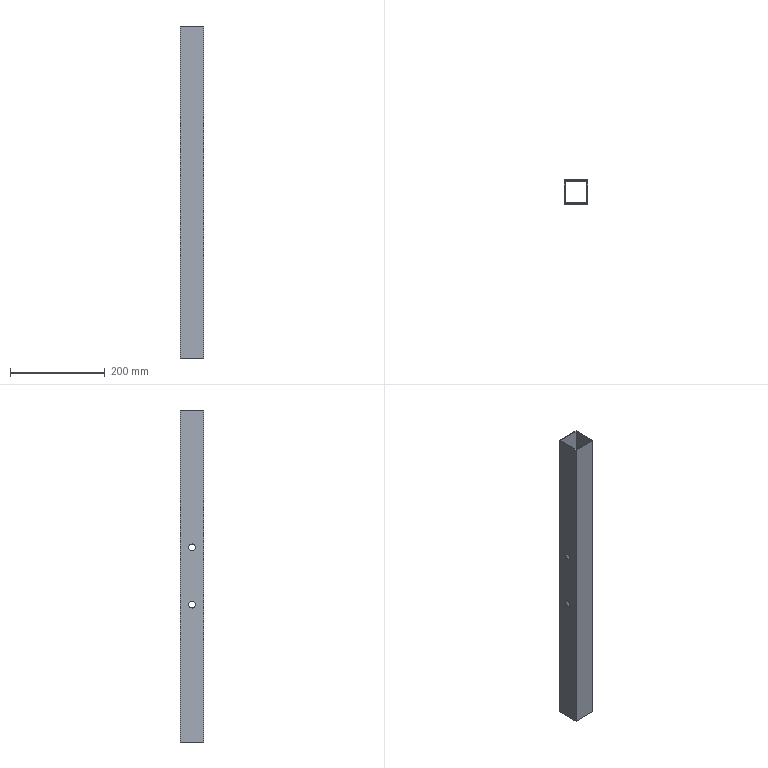Part | SolidWorks | features Extrusion 1, ICE 1 | 1 solid | 18 faces | box 50 x 50 x 700 mm | volume 267568 mm3 | plane 10 | cylinder 8 | commonest cylinder face diameters 14 x8
STEP:
#1=CARTESIAN_POINT('',(25.,0.,403.5));
#2=VERTEX_POINT('',#1);
#3=CARTESIAN_POINT('',(25.,0.,417.5));
#4=VERTEX_POINT('',#3);
#5=CARTESIAN_POINT('',(25.,0.,410.5));
#6=DIRECTION('',(-1.,0.,0.));
#7=DIRECTION('',(0.,0.,-1.));
#8=AXIS2_PLACEMENT_3D('',#5,#6,#7);
#9=CIRCLE('',#8,7.);
#10=EDGE_CURVE('',#2,#4,#9,.T.);
#11=ORIENTED_EDGE('',*,*,#10,.F.);
#12=CARTESIAN_POINT('',(23.,0.,403.5));
#13=VERTEX_POINT('',#12);
#14=CARTESIAN_POINT('',(25.,0.,403.5));
#15=DIRECTION('',(-1.,0.,0.));
#16=VECTOR('',#15,1000.);
#17=LINE('',#14,#16);
#18=EDGE_CURVE('',#2,#13,#17,.T.);
#19=ORIENTED_EDGE('',*,*,#18,.T.);
#20=CARTESIAN_POINT('',(23.,0.,417.5));
#21=VERTEX_POINT('',#20);
#22=CARTESIAN_POINT('',(23.,0.,410.5));
#23=DIRECTION('',(-1.,0.,0.));
#24=DIRECTION('',(0.,0.,1.));
#25=AXIS2_PLACEMENT_3D('',#22,#23,#24);
#26=CIRCLE('',#25,7.);
#27=EDGE_CURVE('',#13,#21,#26,.T.);
#28=ORIENTED_EDGE('',*,*,#27,.T.);
#29=CARTESIAN_POINT('',(25.,0.,417.5));
#30=DIRECTION('',(-1.,0.,0.));
#31=VECTOR('',#30,1000.);
#32=LINE('',#29,#31);
#33=EDGE_CURVE('',#4,#21,#32,.T.);
#34=ORIENTED_EDGE('',*,*,#33,.F.);
#35=EDGE_LOOP('',(#11,#19,#28,#34));
#36=FACE_OUTER_BOUND('',#35,.T.);
#37=CARTESIAN_POINT('',(25.,0.,410.5));
#38=DIRECTION('',(-1.,0.,0.));
#39=DIRECTION('',(0.,0.,1.));
#40=AXIS2_PLACEMENT_3D('',#37,#38,#39);
#41=CYLINDRICAL_SURFACE('',#40,7.);
#42=ADVANCED_FACE('',(#36),#41,.F.);
#43=CARTESIAN_POINT('',(-23.,0.,417.5));
#44=VERTEX_POINT('',#43);
#45=CARTESIAN_POINT('',(-23.,0.,403.5));
#46=VERTEX_POINT('',#45);
#47=CARTESIAN_POINT('',(-23.,0.,410.5));
#48=DIRECTION('',(1.,0.,0.));
#49=DIRECTION('',(0.,0.,-1.));
#50=AXIS2_PLACEMENT_3D('',#47,#48,#49);
#51=CIRCLE('',#50,7.);
#52=EDGE_CURVE('',#44,#46,#51,.T.);
#53=ORIENTED_EDGE('',*,*,#52,.T.);
#54=CARTESIAN_POINT('',(-25.,0.,403.5));
#55=VERTEX_POINT('',#54);
#56=CARTESIAN_POINT('',(25.,0.,403.5));
#57=DIRECTION('',(-1.,0.,0.));
#58=VECTOR('',#57,1000.);
#59=LINE('',#56,#58);
#60=EDGE_CURVE('',#46,#55,#59,.T.);
#61=ORIENTED_EDGE('',*,*,#60,.T.);
#62=CARTESIAN_POINT('',(-25.,0.,417.5));
#63=VERTEX_POINT('',#62);
#64=CARTESIAN_POINT('',(-25.,0.,410.5));
#65=DIRECTION('',(-1.,0.,0.));
#66=DIRECTION('',(0.,0.,-1.));
#67=AXIS2_PLACEMENT_3D('',#64,#65,#66);
#68=CIRCLE('',#67,7.);
#69=EDGE_CURVE('',#55,#63,#68,.T.);
#70=ORIENTED_EDGE('',*,*,#69,.T.);
#71=CARTESIAN_POINT('',(25.,0.,417.5));
#72=DIRECTION('',(-1.,0.,0.));
#73=VECTOR('',#72,1000.);
#74=LINE('',#71,#73);
#75=EDGE_CURVE('',#44,#63,#74,.T.);
#76=ORIENTED_EDGE('',*,*,#75,.F.);
#77=EDGE_LOOP('',(#53,#61,#70,#76));
#78=FACE_OUTER_BOUND('',#77,.T.);
#79=CARTESIAN_POINT('',(25.,0.,410.5));
#80=DIRECTION('',(-1.,0.,0.));
#81=DIRECTION('',(0.,0.,1.));
#82=AXIS2_PLACEMENT_3D('',#79,#80,#81);
#83=CYLINDRICAL_SURFACE('',#82,7.);
#84=ADVANCED_FACE('',(#78),#83,.F.);
#85=CARTESIAN_POINT('',(25.,0.,282.5));
#86=VERTEX_POINT('',#85);
#87=CARTESIAN_POINT('',(25.,0.,296.5));
#88=VERTEX_POINT('',#87);
#89=CARTESIAN_POINT('',(25.,0.,289.5));
#90=DIRECTION('',(-1.,0.,0.));
#91=DIRECTION('',(0.,0.,1.));
#92=AXIS2_PLACEMENT_3D('',#89,#90,#91);
#93=CIRCLE('',#92,7.);
#94=EDGE_CURVE('',#86,#88,#93,.T.);
#95=ORIENTED_EDGE('',*,*,#94,.F.);
#96=CARTESIAN_POINT('',(23.,0.,282.5));
#97=VERTEX_POINT('',#96);
#98=CARTESIAN_POINT('',(25.,0.,282.5));
#99=DIRECTION('',(-1.,0.,0.));
#100=VECTOR('',#99,1000.);
#101=LINE('',#98,#100);
#102=EDGE_CURVE('',#86,#97,#101,.T.);
#103=ORIENTED_EDGE('',*,*,#102,.T.);
#104=CARTESIAN_POINT('',(23.,0.,296.5));
#105=VERTEX_POINT('',#104);
#106=CARTESIAN_POINT('',(23.,0.,289.5));
#107=DIRECTION('',(-1.,0.,0.));
#108=DIRECTION('',(0.,0.,1.));
#109=AXIS2_PLACEMENT_3D('',#106,#107,#108);
#110=CIRCLE('',#109,7.);
#111=EDGE_CURVE('',#97,#105,#110,.T.);
#112=ORIENTED_EDGE('',*,*,#111,.T.);
#113=CARTESIAN_POINT('',(25.,0.,296.5));
#114=DIRECTION('',(-1.,0.,0.));
#115=VECTOR('',#114,1000.);
#116=LINE('',#113,#115);
#117=EDGE_CURVE('',#88,#105,#116,.T.);
#118=ORIENTED_EDGE('',*,*,#117,.F.);
#119=EDGE_LOOP('',(#95,#103,#112,#118));
#120=FACE_OUTER_BOUND('',#119,.T.);
#121=CARTESIAN_POINT('',(25.,0.,289.5));
#122=DIRECTION('',(-1.,0.,0.));
#123=DIRECTION('',(0.,0.,1.));
#124=AXIS2_PLACEMENT_3D('',#121,#122,#123);
#125=CYLINDRICAL_SURFACE('',#124,7.);
#126=ADVANCED_FACE('',(#120),#125,.F.);
#127=CARTESIAN_POINT('',(-23.,0.,296.5));
#128=VERTEX_POINT('',#127);
#129=CARTESIAN_POINT('',(-23.,0.,282.5));
#130=VERTEX_POINT('',#129);
#131=CARTESIAN_POINT('',(-23.,0.,289.5));
#132=DIRECTION('',(1.,0.,0.));
#133=DIRECTION('',(0.,0.,-1.));
#134=AXIS2_PLACEMENT_3D('',#131,#132,#133);
#135=CIRCLE('',#134,7.);
#136=EDGE_CURVE('',#128,#130,#135,.T.);
#137=ORIENTED_EDGE('',*,*,#136,.T.);
#138=CARTESIAN_POINT('',(-25.,0.,282.5));
#139=VERTEX_POINT('',#138);
#140=CARTESIAN_POINT('',(25.,0.,282.5));
#141=DIRECTION('',(-1.,0.,0.));
#142=VECTOR('',#141,1000.);
#143=LINE('',#140,#142);
#144=EDGE_CURVE('',#130,#139,#143,.T.);
#145=ORIENTED_EDGE('',*,*,#144,.T.);
#146=CARTESIAN_POINT('',(-25.,0.,296.5));
#147=VERTEX_POINT('',#146);
#148=CARTESIAN_POINT('',(-25.,0.,289.5));
#149=DIRECTION('',(-1.,0.,0.));
#150=DIRECTION('',(0.,0.,1.));
#151=AXIS2_PLACEMENT_3D('',#148,#149,#150);
#152=CIRCLE('',#151,7.);
#153=EDGE_CURVE('',#139,#147,#152,.T.);
#154=ORIENTED_EDGE('',*,*,#153,.T.);
#155=CARTESIAN_POINT('',(25.,0.,296.5));
#156=DIRECTION('',(-1.,0.,0.));
#157=VECTOR('',#156,1000.);
#158=LINE('',#155,#157);
#159=EDGE_CURVE('',#128,#147,#158,.T.);
#160=ORIENTED_EDGE('',*,*,#159,.F.);
#161=EDGE_LOOP('',(#137,#145,#154,#160));
#162=FACE_OUTER_BOUND('',#161,.T.);
#163=CARTESIAN_POINT('',(25.,0.,289.5));
#164=DIRECTION('',(-1.,0.,0.));
#165=DIRECTION('',(0.,0.,1.));
#166=AXIS2_PLACEMENT_3D('',#163,#164,#165);
#167=CYLINDRICAL_SURFACE('',#166,7.);
#168=ADVANCED_FACE('',(#162),#167,.F.);
#169=CARTESIAN_POINT('',(25.,-25.,700.));
#170=VERTEX_POINT('',#169);
#171=CARTESIAN_POINT('',(25.,25.,700.));
#172=VERTEX_POINT('',#171);
#173=CARTESIAN_POINT('',(25.,-25.,700.));
#174=DIRECTION('',(0.,1.,0.));
#175=VECTOR('',#174,1000.);
#176=LINE('',#173,#175);
#177=EDGE_CURVE('',#170,#172,#176,.T.);
#178=ORIENTED_EDGE('',*,*,#177,.T.);
#179=CARTESIAN_POINT('',(-25.,25.,700.));
#180=VERTEX_POINT('',#179);
#181=CARTESIAN_POINT('',(-25.,25.,700.));
#182=DIRECTION('',(-1.,0.,0.));
#183=VECTOR('',#182,1000.);
#184=LINE('',#181,#183);
#185=EDGE_CURVE('',#172,#180,#184,.T.);
#186=ORIENTED_EDGE('',*,*,#185,.T.);
#187=CARTESIAN_POINT('',(-25.,-25.,700.));
#188=VERTEX_POINT('',#187);
#189=CARTESIAN_POINT('',(-25.,-25.,700.));
#190=DIRECTION('',(0.,-1.,0.));
#191=VECTOR('',#190,1000.);
#192=LINE('',#189,#191);
#193=EDGE_CURVE('',#180,#188,#192,.T.);
#194=ORIENTED_EDGE('',*,*,#193,.T.);
#195=CARTESIAN_POINT('',(-25.,-25.,700.));
#196=DIRECTION('',(1.,0.,0.));
#197=VECTOR('',#196,1000.);
#198=LINE('',#195,#197);
#199=EDGE_CURVE('',#188,#170,#198,.T.);
#200=ORIENTED_EDGE('',*,*,#199,.T.);
#201=EDGE_LOOP('',(#178,#186,#194,#200));
#202=FACE_OUTER_BOUND('',#201,.T.);
#203=CARTESIAN_POINT('',(23.,-23.,700.));
#204=VERTEX_POINT('',#203);
#205=CARTESIAN_POINT('',(23.,23.,700.));
#206=VERTEX_POINT('',#205);
#207=CARTESIAN_POINT('',(23.,-23.,700.));
#208=DIRECTION('',(0.,1.,0.));
#209=VECTOR('',#208,1000.);
#210=LINE('',#207,#209);
#211=EDGE_CURVE('',#204,#206,#210,.T.);
#212=ORIENTED_EDGE('',*,*,#211,.F.);
#213=CARTESIAN_POINT('',(-23.,-23.,700.));
#214=VERTEX_POINT('',#213);
#215=CARTESIAN_POINT('',(-23.,-23.,700.));
#216=DIRECTION('',(1.,0.,0.));
#217=VECTOR('',#216,1000.);
#218=LINE('',#215,#217);
#219=EDGE_CURVE('',#214,#204,#218,.T.);
#220=ORIENTED_EDGE('',*,*,#219,.F.);
#221=CARTESIAN_POINT('',(-23.,23.,700.));
#222=VERTEX_POINT('',#221);
#223=CARTESIAN_POINT('',(-23.,-23.,700.));
#224=DIRECTION('',(0.,-1.,0.));
#225=VECTOR('',#224,1000.);
#226=LINE('',#223,#225);
#227=EDGE_CURVE('',#222,#214,#226,.T.);
#228=ORIENTED_EDGE('',*,*,#227,.F.);
#229=CARTESIAN_POINT('',(-23.,23.,700.));
#230=DIRECTION('',(-1.,0.,0.));
#231=VECTOR('',#230,1000.);
#232=LINE('',#229,#231);
#233=EDGE_CURVE('',#206,#222,#232,.T.);
#234=ORIENTED_EDGE('',*,*,#233,.F.);
#235=EDGE_LOOP('',(#212,#220,#228,#234));
#236=FACE_BOUND('',#235,.T.);
#237=CARTESIAN_POINT('',(0.,0.,700.));
#238=DIRECTION('',(0.,0.,-1.));
#239=DIRECTION('',(-1.,0.,0.));
#240=AXIS2_PLACEMENT_3D('',#237,#238,#239);
#241=PLANE('',#240);
#242=ADVANCED_FACE('',(#202,#236),#241,.F.);
#243=CARTESIAN_POINT('',(25.,-25.,0.));
#244=VERTEX_POINT('',#243);
#245=CARTESIAN_POINT('',(25.,25.,0.));
#246=VERTEX_POINT('',#245);
#247=CARTESIAN_POINT('',(25.,-25.,0.));
#248=DIRECTION('',(0.,1.,0.));
#249=VECTOR('',#248,1000.);
#250=LINE('',#247,#249);
#251=EDGE_CURVE('',#244,#246,#250,.T.);
#252=ORIENTED_EDGE('',*,*,#251,.F.);
#253=CARTESIAN_POINT('',(-25.,-25.,0.));
#254=VERTEX_POINT('',#253);
#255=CARTESIAN_POINT('',(-25.,-25.,0.));
#256=DIRECTION('',(1.,0.,0.));
#257=VECTOR('',#256,1000.);
#258=LINE('',#255,#257);
#259=EDGE_CURVE('',#254,#244,#258,.T.);
#260=ORIENTED_EDGE('',*,*,#259,.F.);
#261=CARTESIAN_POINT('',(-25.,25.,0.));
#262=VERTEX_POINT('',#261);
#263=CARTESIAN_POINT('',(-25.,-25.,0.));
#264=DIRECTION('',(0.,-1.,0.));
#265=VECTOR('',#264,1000.);
#266=LINE('',#263,#265);
#267=EDGE_CURVE('',#262,#254,#266,.T.);
#268=ORIENTED_EDGE('',*,*,#267,.F.);
#269=CARTESIAN_POINT('',(-25.,25.,0.));
#270=DIRECTION('',(-1.,0.,0.));
#271=VECTOR('',#270,1000.);
#272=LINE('',#269,#271);
#273=EDGE_CURVE('',#246,#262,#272,.T.);
#274=ORIENTED_EDGE('',*,*,#273,.F.);
#275=EDGE_LOOP('',(#252,#260,#268,#274));
#276=FACE_OUTER_BOUND('',#275,.T.);
#277=CARTESIAN_POINT('',(-23.,-23.,0.));
#278=VERTEX_POINT('',#277);
#279=CARTESIAN_POINT('',(23.,-23.,0.));
#280=VERTEX_POINT('',#279);
#281=CARTESIAN_POINT('',(-23.,-23.,0.));
#282=DIRECTION('',(1.,0.,0.));
#283=VECTOR('',#282,1000.);
#284=LINE('',#281,#283);
#285=EDGE_CURVE('',#278,#280,#284,.T.);
#286=ORIENTED_EDGE('',*,*,#285,.T.);
#287=CARTESIAN_POINT('',(23.,23.,0.));
#288=VERTEX_POINT('',#287);
#289=CARTESIAN_POINT('',(23.,-23.,0.));
#290=DIRECTION('',(0.,1.,0.));
#291=VECTOR('',#290,1000.);
#292=LINE('',#289,#291);
#293=EDGE_CURVE('',#280,#288,#292,.T.);
#294=ORIENTED_EDGE('',*,*,#293,.T.);
#295=CARTESIAN_POINT('',(-23.,23.,0.));
#296=VERTEX_POINT('',#295);
#297=CARTESIAN_POINT('',(-23.,23.,0.));
#298=DIRECTION('',(-1.,0.,0.));
#299=VECTOR('',#298,1000.);
#300=LINE('',#297,#299);
#301=EDGE_CURVE('',#288,#296,#300,.T.);
#302=ORIENTED_EDGE('',*,*,#301,.T.);
#303=CARTESIAN_POINT('',(-23.,-23.,0.));
#304=DIRECTION('',(0.,-1.,0.));
#305=VECTOR('',#304,1000.);
#306=LINE('',#303,#305);
#307=EDGE_CURVE('',#296,#278,#306,.T.);
#308=ORIENTED_EDGE('',*,*,#307,.T.);
#309=EDGE_LOOP('',(#286,#294,#302,#308));
#310=FACE_BOUND('',#309,.T.);
#311=CARTESIAN_POINT('',(0.,0.,0.));
#312=DIRECTION('',(0.,0.,-1.));
#313=DIRECTION('',(-1.,0.,0.));
#314=AXIS2_PLACEMENT_3D('',#311,#312,#313);
#315=PLANE('',#314);
#316=ADVANCED_FACE('',(#276,#310),#315,.T.);
#317=CARTESIAN_POINT('',(25.,0.,410.5));
#318=DIRECTION('',(-1.,0.,0.));
#319=DIRECTION('',(0.,0.,-1.));
#320=AXIS2_PLACEMENT_3D('',#317,#318,#319);
#321=CIRCLE('',#320,7.);
#322=EDGE_CURVE('',#4,#2,#321,.T.);
#323=ORIENTED_EDGE('',*,*,#322,.T.);
#324=ORIENTED_EDGE('',*,*,#10,.T.);
#325=EDGE_LOOP('',(#323,#324));
#326=FACE_BOUND('',#325,.T.);
#327=CARTESIAN_POINT('',(25.,0.,289.5));
#328=DIRECTION('',(-1.,0.,0.));
#329=DIRECTION('',(0.,0.,1.));
#330=AXIS2_PLACEMENT_3D('',#327,#328,#329);
#331=CIRCLE('',#330,7.);
#332=EDGE_CURVE('',#88,#86,#331,.T.);
#333=ORIENTED_EDGE('',*,*,#332,.T.);
#334=ORIENTED_EDGE('',*,*,#94,.T.);
#335=EDGE_LOOP('',(#333,#334));
#336=FACE_BOUND('',#335,.T.);
#337=ORIENTED_EDGE('',*,*,#251,.T.);
#338=CARTESIAN_POINT('',(25.,25.,700.));
#339=DIRECTION('',(0.,0.,-1.));
#340=VECTOR('',#339,1000.);
#341=LINE('',#338,#340);
#342=EDGE_CURVE('',#172,#246,#341,.T.);
#343=ORIENTED_EDGE('',*,*,#342,.F.);
#344=ORIENTED_EDGE('',*,*,#177,.F.);
#345=CARTESIAN_POINT('',(25.,-25.,700.));
#346=DIRECTION('',(0.,0.,-1.));
#347=VECTOR('',#346,1000.);
#348=LINE('',#345,#347);
#349=EDGE_CURVE('',#170,#244,#348,.T.);
#350=ORIENTED_EDGE('',*,*,#349,.T.);
#351=EDGE_LOOP('',(#337,#343,#344,#350));
#352=FACE_OUTER_BOUND('',#351,.T.);
#353=CARTESIAN_POINT('',(25.,-25.,700.));
#354=DIRECTION('',(-1.,0.,0.));
#355=DIRECTION('',(0.,0.,1.));
#356=AXIS2_PLACEMENT_3D('',#353,#354,#355);
#357=PLANE('',#356);
#358=ADVANCED_FACE('',(#326,#336,#352),#357,.F.);
#359=ORIENTED_EDGE('',*,*,#273,.T.);
#360=CARTESIAN_POINT('',(-25.,25.,700.));
#361=DIRECTION('',(0.,0.,-1.));
#362=VECTOR('',#361,1000.);
#363=LINE('',#360,#362);
#364=EDGE_CURVE('',#180,#262,#363,.T.);
#365=ORIENTED_EDGE('',*,*,#364,.F.);
#366=ORIENTED_EDGE('',*,*,#185,.F.);
#367=ORIENTED_EDGE('',*,*,#342,.T.);
#368=EDGE_LOOP('',(#359,#365,#366,#367));
#369=FACE_OUTER_BOUND('',#368,.T.);
#370=CARTESIAN_POINT('',(-25.,25.,700.));
#371=DIRECTION('',(0.,-1.,0.));
#372=DIRECTION('',(0.,0.,-1.));
#373=AXIS2_PLACEMENT_3D('',#370,#371,#372);
#374=PLANE('',#373);
#375=ADVANCED_FACE('',(#369),#374,.F.);
#376=CARTESIAN_POINT('',(-25.,0.,410.5));
#377=DIRECTION('',(-1.,0.,0.));
#378=DIRECTION('',(0.,0.,-1.));
#379=AXIS2_PLACEMENT_3D('',#376,#377,#378);
#380=CIRCLE('',#379,7.);
#381=EDGE_CURVE('',#63,#55,#380,.T.);
#382=ORIENTED_EDGE('',*,*,#381,.F.);
#383=ORIENTED_EDGE('',*,*,#69,.F.);
#384=EDGE_LOOP('',(#382,#383));
#385=FACE_BOUND('',#384,.T.);
#386=CARTESIAN_POINT('',(-25.,0.,289.5));
#387=DIRECTION('',(-1.,0.,0.));
#388=DIRECTION('',(0.,0.,1.));
#389=AXIS2_PLACEMENT_3D('',#386,#387,#388);
#390=CIRCLE('',#389,7.);
#391=EDGE_CURVE('',#147,#139,#390,.T.);
#392=ORIENTED_EDGE('',*,*,#391,.F.);
#393=ORIENTED_EDGE('',*,*,#153,.F.);
#394=EDGE_LOOP('',(#392,#393));
#395=FACE_BOUND('',#394,.T.);
#396=ORIENTED_EDGE('',*,*,#267,.T.);
#397=CARTESIAN_POINT('',(-25.,-25.,700.));
#398=DIRECTION('',(0.,0.,-1.));
#399=VECTOR('',#398,1000.);
#400=LINE('',#397,#399);
#401=EDGE_CURVE('',#188,#254,#400,.T.);
#402=ORIENTED_EDGE('',*,*,#401,.F.);
#403=ORIENTED_EDGE('',*,*,#193,.F.);
#404=ORIENTED_EDGE('',*,*,#364,.T.);
#405=EDGE_LOOP('',(#396,#402,#403,#404));
#406=FACE_OUTER_BOUND('',#405,.T.);
#407=CARTESIAN_POINT('',(-25.,-25.,700.));
#408=DIRECTION('',(1.,0.,0.));
#409=DIRECTION('',(0.,0.,-1.));
#410=AXIS2_PLACEMENT_3D('',#407,#408,#409);
#411=PLANE('',#410);
#412=ADVANCED_FACE('',(#385,#395,#406),#411,.F.);
#413=ORIENTED_EDGE('',*,*,#259,.T.);
#414=ORIENTED_EDGE('',*,*,#349,.F.);
#415=ORIENTED_EDGE('',*,*,#199,.F.);
#416=ORIENTED_EDGE('',*,*,#401,.T.);
#417=EDGE_LOOP('',(#413,#414,#415,#416));
#418=FACE_OUTER_BOUND('',#417,.T.);
#419=CARTESIAN_POINT('',(-25.,-25.,700.));
#420=DIRECTION('',(0.,1.,0.));
#421=DIRECTION('',(0.,0.,1.));
#422=AXIS2_PLACEMENT_3D('',#419,#420,#421);
#423=PLANE('',#422);
#424=ADVANCED_FACE('',(#418),#423,.F.);
#425=CARTESIAN_POINT('',(23.,0.,410.5));
#426=DIRECTION('',(-1.,0.,0.));
#427=DIRECTION('',(0.,0.,1.));
#428=AXIS2_PLACEMENT_3D('',#425,#426,#427);
#429=CIRCLE('',#428,7.);
#430=EDGE_CURVE('',#21,#13,#429,.T.);
#431=ORIENTED_EDGE('',*,*,#430,.F.);
#432=ORIENTED_EDGE('',*,*,#27,.F.);
#433=EDGE_LOOP('',(#431,#432));
#434=FACE_BOUND('',#433,.T.);
#435=CARTESIAN_POINT('',(23.,0.,289.5));
#436=DIRECTION('',(-1.,0.,0.));
#437=DIRECTION('',(0.,0.,1.));
#438=AXIS2_PLACEMENT_3D('',#435,#436,#437);
#439=CIRCLE('',#438,7.);
#440=EDGE_CURVE('',#105,#97,#439,.T.);
#441=ORIENTED_EDGE('',*,*,#440,.F.);
#442=ORIENTED_EDGE('',*,*,#111,.F.);
#443=EDGE_LOOP('',(#441,#442));
#444=FACE_BOUND('',#443,.T.);
#445=ORIENTED_EDGE('',*,*,#293,.F.);
#446=CARTESIAN_POINT('',(23.,-23.,700.));
#447=DIRECTION('',(0.,0.,-1.));
#448=VECTOR('',#447,1000.);
#449=LINE('',#446,#448);
#450=EDGE_CURVE('',#204,#280,#449,.T.);
#451=ORIENTED_EDGE('',*,*,#450,.F.);
#452=ORIENTED_EDGE('',*,*,#211,.T.);
#453=CARTESIAN_POINT('',(23.,23.,700.));
#454=DIRECTION('',(0.,0.,-1.));
#455=VECTOR('',#454,1000.);
#456=LINE('',#453,#455);
#457=EDGE_CURVE('',#206,#288,#456,.T.);
#458=ORIENTED_EDGE('',*,*,#457,.T.);
#459=EDGE_LOOP('',(#445,#451,#452,#458));
#460=FACE_OUTER_BOUND('',#459,.T.);
#461=CARTESIAN_POINT('',(23.,-23.,700.));
#462=DIRECTION('',(-1.,0.,0.));
#463=DIRECTION('',(0.,0.,1.));
#464=AXIS2_PLACEMENT_3D('',#461,#462,#463);
#465=PLANE('',#464);
#466=ADVANCED_FACE('',(#434,#444,#460),#465,.T.);
#467=ORIENTED_EDGE('',*,*,#301,.F.);
#468=ORIENTED_EDGE('',*,*,#457,.F.);
#469=ORIENTED_EDGE('',*,*,#233,.T.);
#470=CARTESIAN_POINT('',(-23.,23.,700.));
#471=DIRECTION('',(0.,0.,-1.));
#472=VECTOR('',#471,1000.);
#473=LINE('',#470,#472);
#474=EDGE_CURVE('',#222,#296,#473,.T.);
#475=ORIENTED_EDGE('',*,*,#474,.T.);
#476=EDGE_LOOP('',(#467,#468,#469,#475));
#477=FACE_OUTER_BOUND('',#476,.T.);
#478=CARTESIAN_POINT('',(-23.,23.,700.));
#479=DIRECTION('',(0.,-1.,0.));
#480=DIRECTION('',(0.,0.,-1.));
#481=AXIS2_PLACEMENT_3D('',#478,#479,#480);
#482=PLANE('',#481);
#483=ADVANCED_FACE('',(#477),#482,.T.);
#484=ORIENTED_EDGE('',*,*,#52,.F.);
#485=CARTESIAN_POINT('',(-23.,0.,410.5));
#486=DIRECTION('',(1.,0.,0.));
#487=DIRECTION('',(0.,0.,-1.));
#488=AXIS2_PLACEMENT_3D('',#485,#486,#487);
#489=CIRCLE('',#488,7.);
#490=EDGE_CURVE('',#46,#44,#489,.T.);
#491=ORIENTED_EDGE('',*,*,#490,.F.);
#492=EDGE_LOOP('',(#484,#491));
#493=FACE_BOUND('',#492,.T.);
#494=ORIENTED_EDGE('',*,*,#136,.F.);
#495=CARTESIAN_POINT('',(-23.,0.,289.5));
#496=DIRECTION('',(1.,0.,0.));
#497=DIRECTION('',(0.,0.,-1.));
#498=AXIS2_PLACEMENT_3D('',#495,#496,#497);
#499=CIRCLE('',#498,7.);
#500=EDGE_CURVE('',#130,#128,#499,.T.);
#501=ORIENTED_EDGE('',*,*,#500,.F.);
#502=EDGE_LOOP('',(#494,#501));
#503=FACE_BOUND('',#502,.T.);
#504=ORIENTED_EDGE('',*,*,#307,.F.);
#505=ORIENTED_EDGE('',*,*,#474,.F.);
#506=ORIENTED_EDGE('',*,*,#227,.T.);
#507=CARTESIAN_POINT('',(-23.,-23.,700.));
#508=DIRECTION('',(0.,0.,-1.));
#509=VECTOR('',#508,1000.);
#510=LINE('',#507,#509);
#511=EDGE_CURVE('',#214,#278,#510,.T.);
#512=ORIENTED_EDGE('',*,*,#511,.T.);
#513=EDGE_LOOP('',(#504,#505,#506,#512));
#514=FACE_OUTER_BOUND('',#513,.T.);
#515=CARTESIAN_POINT('',(-23.,-23.,700.));
#516=DIRECTION('',(1.,0.,0.));
#517=DIRECTION('',(0.,0.,-1.));
#518=AXIS2_PLACEMENT_3D('',#515,#516,#517);
#519=PLANE('',#518);
#520=ADVANCED_FACE('',(#493,#503,#514),#519,.T.);
#521=ORIENTED_EDGE('',*,*,#285,.F.);
#522=ORIENTED_EDGE('',*,*,#511,.F.);
#523=ORIENTED_EDGE('',*,*,#219,.T.);
#524=ORIENTED_EDGE('',*,*,#450,.T.);
#525=EDGE_LOOP('',(#521,#522,#523,#524));
#526=FACE_OUTER_BOUND('',#525,.T.);
#527=CARTESIAN_POINT('',(-23.,-23.,700.));
#528=DIRECTION('',(0.,1.,0.));
#529=DIRECTION('',(0.,0.,1.));
#530=AXIS2_PLACEMENT_3D('',#527,#528,#529);
#531=PLANE('',#530);
#532=ADVANCED_FACE('',(#526),#531,.T.);
#533=ORIENTED_EDGE('',*,*,#144,.F.);
#534=ORIENTED_EDGE('',*,*,#500,.T.);
#535=ORIENTED_EDGE('',*,*,#159,.T.);
#536=ORIENTED_EDGE('',*,*,#391,.T.);
#537=EDGE_LOOP('',(#533,#534,#535,#536));
#538=FACE_OUTER_BOUND('',#537,.T.);
#539=CARTESIAN_POINT('',(25.,0.,289.5));
#540=DIRECTION('',(-1.,0.,0.));
#541=DIRECTION('',(0.,0.,1.));
#542=AXIS2_PLACEMENT_3D('',#539,#540,#541);
#543=CYLINDRICAL_SURFACE('',#542,7.);
#544=ADVANCED_FACE('',(#538),#543,.F.);
#545=ORIENTED_EDGE('',*,*,#102,.F.);
#546=ORIENTED_EDGE('',*,*,#332,.F.);
#547=ORIENTED_EDGE('',*,*,#117,.T.);
#548=ORIENTED_EDGE('',*,*,#440,.T.);
#549=EDGE_LOOP('',(#545,#546,#547,#548));
#550=FACE_OUTER_BOUND('',#549,.T.);
#551=CARTESIAN_POINT('',(25.,0.,289.5));
#552=DIRECTION('',(-1.,0.,0.));
#553=DIRECTION('',(0.,0.,1.));
#554=AXIS2_PLACEMENT_3D('',#551,#552,#553);
#555=CYLINDRICAL_SURFACE('',#554,7.);
#556=ADVANCED_FACE('',(#550),#555,.F.);
#557=ORIENTED_EDGE('',*,*,#60,.F.);
#558=ORIENTED_EDGE('',*,*,#490,.T.);
#559=ORIENTED_EDGE('',*,*,#75,.T.);
#560=ORIENTED_EDGE('',*,*,#381,.T.);
#561=EDGE_LOOP('',(#557,#558,#559,#560));
#562=FACE_OUTER_BOUND('',#561,.T.);
#563=CARTESIAN_POINT('',(25.,0.,410.5));
#564=DIRECTION('',(-1.,0.,0.));
#565=DIRECTION('',(0.,0.,1.));
#566=AXIS2_PLACEMENT_3D('',#563,#564,#565);
#567=CYLINDRICAL_SURFACE('',#566,7.);
#568=ADVANCED_FACE('',(#562),#567,.F.);
#569=ORIENTED_EDGE('',*,*,#18,.F.);
#570=ORIENTED_EDGE('',*,*,#322,.F.);
#571=ORIENTED_EDGE('',*,*,#33,.T.);
#572=ORIENTED_EDGE('',*,*,#430,.T.);
#573=EDGE_LOOP('',(#569,#570,#571,#572));
#574=FACE_OUTER_BOUND('',#573,.T.);
#575=CARTESIAN_POINT('',(25.,0.,410.5));
#576=DIRECTION('',(-1.,0.,0.));
#577=DIRECTION('',(0.,0.,1.));
#578=AXIS2_PLACEMENT_3D('',#575,#576,#577);
#579=CYLINDRICAL_SURFACE('',#578,7.);
#580=ADVANCED_FACE('',(#574),#579,.F.);
#581=CLOSED_SHELL('',(#42,#84,#126,#168,#242,#316,#358,#375,#412,#424,#466,#483,#520,#532,#544,#556,#568,#580));
#582=MANIFOLD_SOLID_BREP('',#581);
#583=CARTESIAN_POINT('',(0.,0.,0.));
#584=DIRECTION('',(0.,0.,1.));
#585=DIRECTION('',(1.,0.,0.));
#586=AXIS2_PLACEMENT_3D('',#583,#584,#585);
#587=(LENGTH_UNIT()NAMED_UNIT(*)SI_UNIT(.MILLI.,.METRE.));
#588=UNCERTAINTY_MEASURE_WITH_UNIT(LENGTH_MEASURE(0.00001),#587,'','');
#589=(NAMED_UNIT(*)PLANE_ANGLE_UNIT()SI_UNIT($,.RADIAN.));
#590=(NAMED_UNIT(*)SI_UNIT($,.STERADIAN.)SOLID_ANGLE_UNIT());
#591=(GEOMETRIC_REPRESENTATION_CONTEXT(3)GLOBAL_UNCERTAINTY_ASSIGNED_CONTEXT((#588))GLOBAL_UNIT_ASSIGNED_CONTEXT((#587,#589,#590))REPRESENTATION_CONTEXT('',''));
#592=ADVANCED_BREP_SHAPE_REPRESENTATION('',(#582,#586),#591);